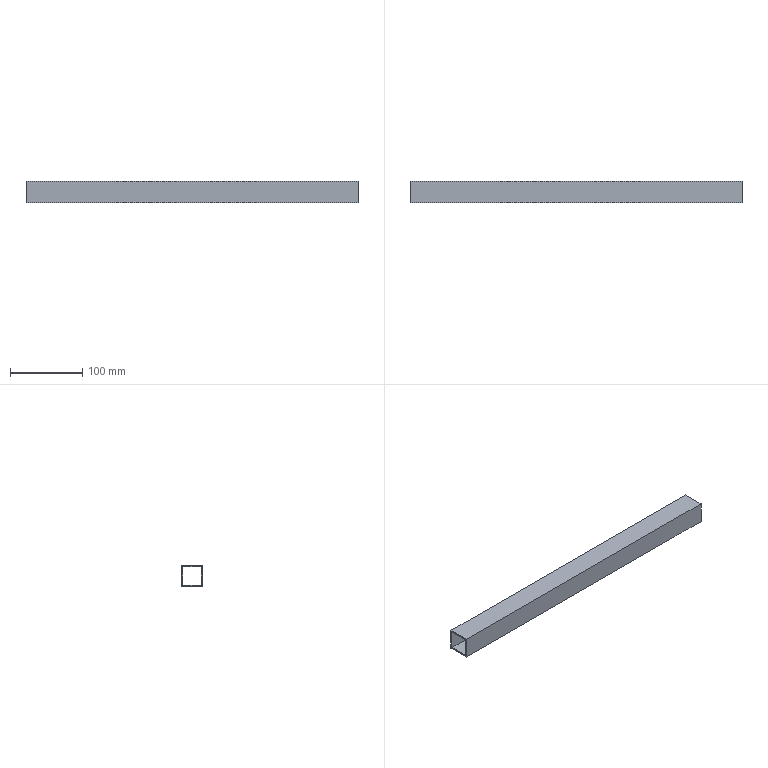Part | NX | features solid 2 | 1 solid | 10 faces | box 460 x 30 x 30 mm | volume 103040 mm3 | plane 10
STEP:
#1=CARTESIAN_POINT('',(250.,-130.,50.));
#2=VERTEX_POINT('',#1);
#3=CARTESIAN_POINT('',(-210.,-130.,50.));
#4=VERTEX_POINT('',#3);
#5=CARTESIAN_POINT('',(200.,-130.,50.));
#6=DIRECTION('',(-1.,0.,0.));
#7=VECTOR('',#6,1000.);
#8=LINE('',#5,#7);
#9=EDGE_CURVE('',#2,#4,#8,.T.);
#10=ORIENTED_EDGE('',*,*,#9,.T.);
#11=CARTESIAN_POINT('',(-210.,-130.,20.));
#12=VERTEX_POINT('',#11);
#13=CARTESIAN_POINT('',(-210.,-130.,50.));
#14=DIRECTION('',(0.,0.,-1.));
#15=VECTOR('',#14,1000.);
#16=LINE('',#13,#15);
#17=EDGE_CURVE('',#4,#12,#16,.T.);
#18=ORIENTED_EDGE('',*,*,#17,.T.);
#19=CARTESIAN_POINT('',(250.,-130.,20.));
#20=VERTEX_POINT('',#19);
#21=CARTESIAN_POINT('',(200.,-130.,20.));
#22=DIRECTION('',(-1.,0.,0.));
#23=VECTOR('',#22,1000.);
#24=LINE('',#21,#23);
#25=EDGE_CURVE('',#20,#12,#24,.T.);
#26=ORIENTED_EDGE('',*,*,#25,.F.);
#27=CARTESIAN_POINT('',(250.,-130.,50.));
#28=DIRECTION('',(0.,0.,-1.));
#29=VECTOR('',#28,1000.);
#30=LINE('',#27,#29);
#31=EDGE_CURVE('',#2,#20,#30,.T.);
#32=ORIENTED_EDGE('',*,*,#31,.F.);
#33=EDGE_LOOP('',(#10,#18,#26,#32));
#34=FACE_BOUND('',#33,.T.);
#35=CARTESIAN_POINT('',(200.,-130.,50.));
#36=DIRECTION('',(0.,-1.,0.));
#37=DIRECTION('',(0.,0.,-1.));
#38=AXIS2_PLACEMENT_3D('',#35,#36,#37);
#39=PLANE('',#38);
#40=ADVANCED_FACE('',(#34),#39,.T.);
#41=CARTESIAN_POINT('',(-210.,-100.,50.));
#42=VERTEX_POINT('',#41);
#43=CARTESIAN_POINT('',(-210.,-100.,20.));
#44=VERTEX_POINT('',#43);
#45=CARTESIAN_POINT('',(-210.,-100.,50.));
#46=DIRECTION('',(0.,0.,-1.));
#47=VECTOR('',#46,1000.);
#48=LINE('',#45,#47);
#49=EDGE_CURVE('',#42,#44,#48,.T.);
#50=ORIENTED_EDGE('',*,*,#49,.F.);
#51=CARTESIAN_POINT('',(250.,-100.,50.));
#52=VERTEX_POINT('',#51);
#53=CARTESIAN_POINT('',(200.,-100.,50.));
#54=DIRECTION('',(-1.,0.,0.));
#55=VECTOR('',#54,1000.);
#56=LINE('',#53,#55);
#57=EDGE_CURVE('',#52,#42,#56,.T.);
#58=ORIENTED_EDGE('',*,*,#57,.F.);
#59=CARTESIAN_POINT('',(250.,-100.,20.));
#60=VERTEX_POINT('',#59);
#61=CARTESIAN_POINT('',(250.,-100.,50.));
#62=DIRECTION('',(0.,0.,-1.));
#63=VECTOR('',#62,1000.);
#64=LINE('',#61,#63);
#65=EDGE_CURVE('',#52,#60,#64,.T.);
#66=ORIENTED_EDGE('',*,*,#65,.T.);
#67=CARTESIAN_POINT('',(200.,-100.,20.));
#68=DIRECTION('',(-1.,0.,0.));
#69=VECTOR('',#68,1000.);
#70=LINE('',#67,#69);
#71=EDGE_CURVE('',#60,#44,#70,.T.);
#72=ORIENTED_EDGE('',*,*,#71,.T.);
#73=EDGE_LOOP('',(#50,#58,#66,#72));
#74=FACE_BOUND('',#73,.T.);
#75=CARTESIAN_POINT('',(200.,-100.,50.));
#76=DIRECTION('',(0.,-1.,0.));
#77=DIRECTION('',(0.,0.,-1.));
#78=AXIS2_PLACEMENT_3D('',#75,#76,#77);
#79=PLANE('',#78);
#80=ADVANCED_FACE('',(#74),#79,.F.);
#81=CARTESIAN_POINT('',(-210.,-130.,50.));
#82=DIRECTION('',(0.,1.,0.));
#83=VECTOR('',#82,1000.);
#84=LINE('',#81,#83);
#85=EDGE_CURVE('',#4,#42,#84,.T.);
#86=ORIENTED_EDGE('',*,*,#85,.F.);
#87=ORIENTED_EDGE('',*,*,#9,.F.);
#88=CARTESIAN_POINT('',(250.,-130.,50.));
#89=DIRECTION('',(0.,-1.,0.));
#90=VECTOR('',#89,1000.);
#91=LINE('',#88,#90);
#92=EDGE_CURVE('',#52,#2,#91,.T.);
#93=ORIENTED_EDGE('',*,*,#92,.F.);
#94=ORIENTED_EDGE('',*,*,#57,.T.);
#95=EDGE_LOOP('',(#86,#87,#93,#94));
#96=FACE_BOUND('',#95,.T.);
#97=CARTESIAN_POINT('',(200.,-130.,50.));
#98=DIRECTION('',(0.,0.,-1.));
#99=DIRECTION('',(0.,1.,0.));
#100=AXIS2_PLACEMENT_3D('',#97,#98,#99);
#101=PLANE('',#100);
#102=ADVANCED_FACE('',(#96),#101,.F.);
#103=ORIENTED_EDGE('',*,*,#25,.T.);
#104=CARTESIAN_POINT('',(-210.,-130.,20.));
#105=DIRECTION('',(0.,1.,0.));
#106=VECTOR('',#105,1000.);
#107=LINE('',#104,#106);
#108=EDGE_CURVE('',#12,#44,#107,.T.);
#109=ORIENTED_EDGE('',*,*,#108,.T.);
#110=ORIENTED_EDGE('',*,*,#71,.F.);
#111=CARTESIAN_POINT('',(250.,-130.,20.));
#112=DIRECTION('',(0.,-1.,0.));
#113=VECTOR('',#112,1000.);
#114=LINE('',#111,#113);
#115=EDGE_CURVE('',#60,#20,#114,.T.);
#116=ORIENTED_EDGE('',*,*,#115,.T.);
#117=EDGE_LOOP('',(#103,#109,#110,#116));
#118=FACE_BOUND('',#117,.T.);
#119=CARTESIAN_POINT('',(200.,-130.,20.));
#120=DIRECTION('',(0.,0.,-1.));
#121=DIRECTION('',(0.,1.,0.));
#122=AXIS2_PLACEMENT_3D('',#119,#120,#121);
#123=PLANE('',#122);
#124=ADVANCED_FACE('',(#118),#123,.T.);
#125=CARTESIAN_POINT('',(-210.,-128.,48.));
#126=VERTEX_POINT('',#125);
#127=CARTESIAN_POINT('',(-210.,-128.,22.));
#128=VERTEX_POINT('',#127);
#129=CARTESIAN_POINT('',(-210.,-128.,50.));
#130=DIRECTION('',(0.,0.,-1.));
#131=VECTOR('',#130,1000.);
#132=LINE('',#129,#131);
#133=EDGE_CURVE('',#126,#128,#132,.T.);
#134=ORIENTED_EDGE('',*,*,#133,.F.);
#135=CARTESIAN_POINT('',(250.,-128.,48.));
#136=VERTEX_POINT('',#135);
#137=CARTESIAN_POINT('',(200.,-128.,48.));
#138=DIRECTION('',(-1.,0.,0.));
#139=VECTOR('',#138,1000.);
#140=LINE('',#137,#139);
#141=EDGE_CURVE('',#136,#126,#140,.T.);
#142=ORIENTED_EDGE('',*,*,#141,.F.);
#143=CARTESIAN_POINT('',(250.,-128.,22.));
#144=VERTEX_POINT('',#143);
#145=CARTESIAN_POINT('',(250.,-128.,50.));
#146=DIRECTION('',(0.,0.,-1.));
#147=VECTOR('',#146,1000.);
#148=LINE('',#145,#147);
#149=EDGE_CURVE('',#136,#144,#148,.T.);
#150=ORIENTED_EDGE('',*,*,#149,.T.);
#151=CARTESIAN_POINT('',(200.,-128.,22.));
#152=DIRECTION('',(-1.,0.,0.));
#153=VECTOR('',#152,1000.);
#154=LINE('',#151,#153);
#155=EDGE_CURVE('',#144,#128,#154,.T.);
#156=ORIENTED_EDGE('',*,*,#155,.T.);
#157=EDGE_LOOP('',(#134,#142,#150,#156));
#158=FACE_BOUND('',#157,.T.);
#159=CARTESIAN_POINT('',(200.,-128.,50.));
#160=DIRECTION('',(0.,-1.,0.));
#161=DIRECTION('',(0.,0.,-1.));
#162=AXIS2_PLACEMENT_3D('',#159,#160,#161);
#163=PLANE('',#162);
#164=ADVANCED_FACE('',(#158),#163,.F.);
#165=CARTESIAN_POINT('',(250.,-102.,48.));
#166=VERTEX_POINT('',#165);
#167=CARTESIAN_POINT('',(-210.,-102.,48.));
#168=VERTEX_POINT('',#167);
#169=CARTESIAN_POINT('',(200.,-102.,48.));
#170=DIRECTION('',(-1.,0.,0.));
#171=VECTOR('',#170,1000.);
#172=LINE('',#169,#171);
#173=EDGE_CURVE('',#166,#168,#172,.T.);
#174=ORIENTED_EDGE('',*,*,#173,.T.);
#175=CARTESIAN_POINT('',(-210.,-102.,22.));
#176=VERTEX_POINT('',#175);
#177=CARTESIAN_POINT('',(-210.,-102.,50.));
#178=DIRECTION('',(0.,0.,-1.));
#179=VECTOR('',#178,1000.);
#180=LINE('',#177,#179);
#181=EDGE_CURVE('',#168,#176,#180,.T.);
#182=ORIENTED_EDGE('',*,*,#181,.T.);
#183=CARTESIAN_POINT('',(250.,-102.,22.));
#184=VERTEX_POINT('',#183);
#185=CARTESIAN_POINT('',(200.,-102.,22.));
#186=DIRECTION('',(-1.,0.,0.));
#187=VECTOR('',#186,1000.);
#188=LINE('',#185,#187);
#189=EDGE_CURVE('',#184,#176,#188,.T.);
#190=ORIENTED_EDGE('',*,*,#189,.F.);
#191=CARTESIAN_POINT('',(250.,-102.,50.));
#192=DIRECTION('',(0.,0.,-1.));
#193=VECTOR('',#192,1000.);
#194=LINE('',#191,#193);
#195=EDGE_CURVE('',#166,#184,#194,.T.);
#196=ORIENTED_EDGE('',*,*,#195,.F.);
#197=EDGE_LOOP('',(#174,#182,#190,#196));
#198=FACE_BOUND('',#197,.T.);
#199=CARTESIAN_POINT('',(200.,-102.,50.));
#200=DIRECTION('',(0.,-1.,0.));
#201=DIRECTION('',(0.,0.,-1.));
#202=AXIS2_PLACEMENT_3D('',#199,#200,#201);
#203=PLANE('',#202);
#204=ADVANCED_FACE('',(#198),#203,.T.);
#205=ORIENTED_EDGE('',*,*,#141,.T.);
#206=CARTESIAN_POINT('',(-210.,-130.,48.));
#207=DIRECTION('',(0.,1.,0.));
#208=VECTOR('',#207,1000.);
#209=LINE('',#206,#208);
#210=EDGE_CURVE('',#126,#168,#209,.T.);
#211=ORIENTED_EDGE('',*,*,#210,.T.);
#212=ORIENTED_EDGE('',*,*,#173,.F.);
#213=CARTESIAN_POINT('',(250.,-130.,48.));
#214=DIRECTION('',(0.,-1.,0.));
#215=VECTOR('',#214,1000.);
#216=LINE('',#213,#215);
#217=EDGE_CURVE('',#166,#136,#216,.T.);
#218=ORIENTED_EDGE('',*,*,#217,.T.);
#219=EDGE_LOOP('',(#205,#211,#212,#218));
#220=FACE_BOUND('',#219,.T.);
#221=CARTESIAN_POINT('',(200.,-130.,48.));
#222=DIRECTION('',(0.,0.,-1.));
#223=DIRECTION('',(0.,1.,0.));
#224=AXIS2_PLACEMENT_3D('',#221,#222,#223);
#225=PLANE('',#224);
#226=ADVANCED_FACE('',(#220),#225,.T.);
#227=CARTESIAN_POINT('',(-210.,-130.,22.));
#228=DIRECTION('',(0.,1.,0.));
#229=VECTOR('',#228,1000.);
#230=LINE('',#227,#229);
#231=EDGE_CURVE('',#128,#176,#230,.T.);
#232=ORIENTED_EDGE('',*,*,#231,.F.);
#233=ORIENTED_EDGE('',*,*,#155,.F.);
#234=CARTESIAN_POINT('',(250.,-130.,22.));
#235=DIRECTION('',(0.,-1.,0.));
#236=VECTOR('',#235,1000.);
#237=LINE('',#234,#236);
#238=EDGE_CURVE('',#184,#144,#237,.T.);
#239=ORIENTED_EDGE('',*,*,#238,.F.);
#240=ORIENTED_EDGE('',*,*,#189,.T.);
#241=EDGE_LOOP('',(#232,#233,#239,#240));
#242=FACE_BOUND('',#241,.T.);
#243=CARTESIAN_POINT('',(200.,-130.,22.));
#244=DIRECTION('',(0.,0.,-1.));
#245=DIRECTION('',(0.,1.,0.));
#246=AXIS2_PLACEMENT_3D('',#243,#244,#245);
#247=PLANE('',#246);
#248=ADVANCED_FACE('',(#242),#247,.F.);
#249=ORIENTED_EDGE('',*,*,#115,.F.);
#250=ORIENTED_EDGE('',*,*,#65,.F.);
#251=ORIENTED_EDGE('',*,*,#92,.T.);
#252=ORIENTED_EDGE('',*,*,#31,.T.);
#253=EDGE_LOOP('',(#249,#250,#251,#252));
#254=FACE_BOUND('',#253,.T.);
#255=ORIENTED_EDGE('',*,*,#195,.T.);
#256=ORIENTED_EDGE('',*,*,#238,.T.);
#257=ORIENTED_EDGE('',*,*,#149,.F.);
#258=ORIENTED_EDGE('',*,*,#217,.F.);
#259=EDGE_LOOP('',(#255,#256,#257,#258));
#260=FACE_BOUND('',#259,.T.);
#261=CARTESIAN_POINT('',(250.,-100.,50.));
#262=DIRECTION('',(1.,0.,0.));
#263=DIRECTION('',(0.,0.,1.));
#264=AXIS2_PLACEMENT_3D('',#261,#262,#263);
#265=PLANE('',#264);
#266=ADVANCED_FACE('',(#254,#260),#265,.T.);
#267=ORIENTED_EDGE('',*,*,#210,.F.);
#268=ORIENTED_EDGE('',*,*,#133,.T.);
#269=ORIENTED_EDGE('',*,*,#231,.T.);
#270=ORIENTED_EDGE('',*,*,#181,.F.);
#271=EDGE_LOOP('',(#267,#268,#269,#270));
#272=FACE_BOUND('',#271,.T.);
#273=ORIENTED_EDGE('',*,*,#17,.F.);
#274=ORIENTED_EDGE('',*,*,#85,.T.);
#275=ORIENTED_EDGE('',*,*,#49,.T.);
#276=ORIENTED_EDGE('',*,*,#108,.F.);
#277=EDGE_LOOP('',(#273,#274,#275,#276));
#278=FACE_BOUND('',#277,.T.);
#279=CARTESIAN_POINT('',(-210.,340.,50.));
#280=DIRECTION('',(-1.,0.,0.));
#281=DIRECTION('',(0.,0.,-1.));
#282=AXIS2_PLACEMENT_3D('',#279,#280,#281);
#283=PLANE('',#282);
#284=ADVANCED_FACE('',(#272,#278),#283,.T.);
#285=CLOSED_SHELL('',(#40,#80,#102,#124,#164,#204,#226,#248,#266,#284));
#286=MANIFOLD_SOLID_BREP('',#285);
#287=(LENGTH_UNIT()NAMED_UNIT(*)SI_UNIT(.MILLI.,.METRE.));
#288=UNCERTAINTY_MEASURE_WITH_UNIT(LENGTH_MEASURE(0.00001),#287,'','');
#289=(NAMED_UNIT(*)PLANE_ANGLE_UNIT()SI_UNIT($,.RADIAN.));
#290=(NAMED_UNIT(*)SI_UNIT($,.STERADIAN.)SOLID_ANGLE_UNIT());
#291=(GEOMETRIC_REPRESENTATION_CONTEXT(3)GLOBAL_UNCERTAINTY_ASSIGNED_CONTEXT((#288))GLOBAL_UNIT_ASSIGNED_CONTEXT((#287,#289,#290))REPRESENTATION_CONTEXT('',''));
#292=ADVANCED_BREP_SHAPE_REPRESENTATION('',(#286),#291);